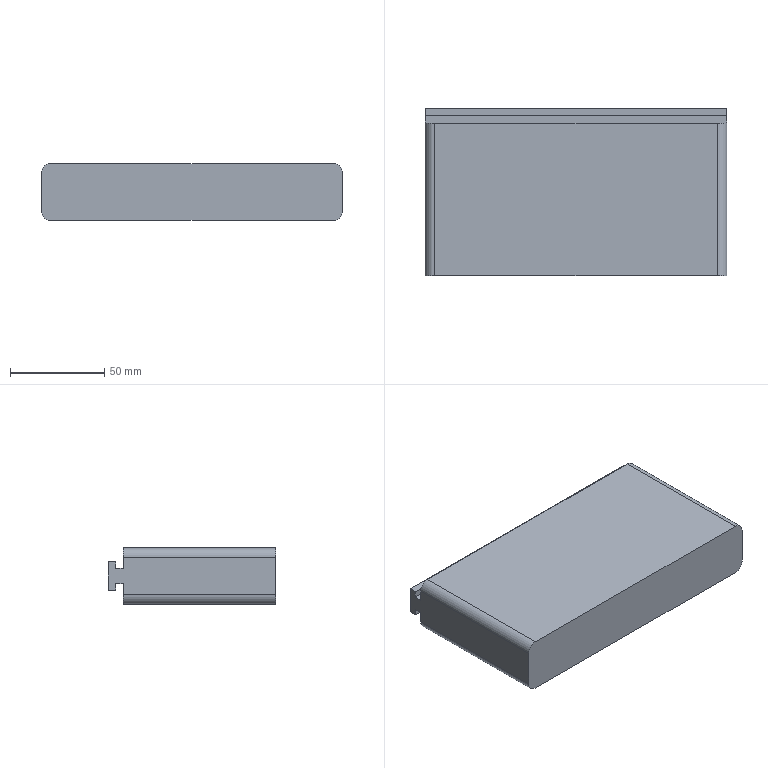Part | STEP file | RACK-BASE2_id654_x_t | 1 solid | 18 faces | box 160 x 89.028 x 30 mm | volume 401916 mm3 | plane 14 | cylinder 4 | commonest cylinder face diameters 10 x4
STEP:
#1=CARTESIAN_POINT('',(-110.,-174.472,83.5));
#2=VERTEX_POINT('',#1);
#3=CARTESIAN_POINT('',(50.,-174.472,83.5));
#4=VERTEX_POINT('',#3);
#5=CARTESIAN_POINT('',(30.,-174.472,83.5));
#6=DIRECTION('',(1.,0.,0.));
#7=VECTOR('',#6,1.);
#8=LINE('',#5,#7);
#9=EDGE_CURVE('',#2,#4,#8,.T.);
#10=ORIENTED_EDGE('',*,*,#9,.T.);
#11=CARTESIAN_POINT('',(50.,-174.472,77.5));
#12=VERTEX_POINT('',#11);
#13=CARTESIAN_POINT('',(50.,-174.472,102.5));
#14=DIRECTION('',(0.,0.,1.));
#15=VECTOR('',#14,1.);
#16=LINE('',#13,#15);
#17=EDGE_CURVE('',#12,#4,#16,.T.);
#18=ORIENTED_EDGE('',*,*,#17,.F.);
#19=CARTESIAN_POINT('',(45.,-174.472,72.5));
#20=VERTEX_POINT('',#19);
#21=CARTESIAN_POINT('',(45.,-174.472,77.5));
#22=DIRECTION('',(0.,-1.,0.));
#23=DIRECTION('',(0.,0.,-1.));
#24=AXIS2_PLACEMENT_3D('',#21,#22,#23);
#25=CIRCLE('',#24,5.);
#26=EDGE_CURVE('',#20,#12,#25,.T.);
#27=ORIENTED_EDGE('',*,*,#26,.F.);
#28=CARTESIAN_POINT('',(-105.,-174.472,72.5));
#29=VERTEX_POINT('',#28);
#30=CARTESIAN_POINT('',(50.126,-174.472,72.5));
#31=DIRECTION('',(1.,0.,0.));
#32=VECTOR('',#31,1.);
#33=LINE('',#30,#32);
#34=EDGE_CURVE('',#29,#20,#33,.T.);
#35=ORIENTED_EDGE('',*,*,#34,.F.);
#36=CARTESIAN_POINT('',(-110.,-174.472,77.5));
#37=VERTEX_POINT('',#36);
#38=CARTESIAN_POINT('',(-105.,-174.472,77.5));
#39=DIRECTION('',(0.,-1.,0.));
#40=DIRECTION('',(0.,0.,1.));
#41=AXIS2_PLACEMENT_3D('',#38,#39,#40);
#42=CIRCLE('',#41,5.);
#43=EDGE_CURVE('',#37,#29,#42,.T.);
#44=ORIENTED_EDGE('',*,*,#43,.F.);
#45=CARTESIAN_POINT('',(-110.,-174.472,102.5));
#46=DIRECTION('',(0.,0.,-1.));
#47=VECTOR('',#46,1.);
#48=LINE('',#45,#47);
#49=EDGE_CURVE('',#2,#37,#48,.T.);
#50=ORIENTED_EDGE('',*,*,#49,.F.);
#51=EDGE_LOOP('',(#10,#18,#27,#35,#44,#50));
#52=FACE_OUTER_BOUND('',#51,.T.);
#53=CARTESIAN_POINT('',(30.,-174.472,83.5));
#54=DIRECTION('',(0.,-1.,0.));
#55=DIRECTION('',(0.,0.,-1.));
#56=AXIS2_PLACEMENT_3D('',#53,#54,#55);
#57=PLANE('',#56);
#58=ADVANCED_FACE('',(#52),#57,.F.);
#59=CARTESIAN_POINT('',(-110.,-170.472,83.5));
#60=VERTEX_POINT('',#59);
#61=CARTESIAN_POINT('',(-110.,-255.5,83.5));
#62=DIRECTION('',(0.,-1.,0.));
#63=VECTOR('',#62,1.);
#64=LINE('',#61,#63);
#65=EDGE_CURVE('',#60,#2,#64,.T.);
#66=ORIENTED_EDGE('',*,*,#65,.F.);
#67=CARTESIAN_POINT('',(50.,-170.472,83.5));
#68=VERTEX_POINT('',#67);
#69=CARTESIAN_POINT('',(30.,-170.472,83.5));
#70=DIRECTION('',(1.,0.,0.));
#71=VECTOR('',#70,1.);
#72=LINE('',#69,#71);
#73=EDGE_CURVE('',#60,#68,#72,.T.);
#74=ORIENTED_EDGE('',*,*,#73,.T.);
#75=CARTESIAN_POINT('',(50.,-166.472,83.5));
#76=DIRECTION('',(0.,1.,0.));
#77=VECTOR('',#76,1.);
#78=LINE('',#75,#77);
#79=EDGE_CURVE('',#4,#68,#78,.T.);
#80=ORIENTED_EDGE('',*,*,#79,.F.);
#81=ORIENTED_EDGE('',*,*,#9,.F.);
#82=EDGE_LOOP('',(#66,#74,#80,#81));
#83=FACE_OUTER_BOUND('',#82,.T.);
#84=CARTESIAN_POINT('',(30.,-170.472,83.5));
#85=DIRECTION('',(0.,0.,1.));
#86=DIRECTION('',(1.,0.,0.));
#87=AXIS2_PLACEMENT_3D('',#84,#85,#86);
#88=PLANE('',#87);
#89=ADVANCED_FACE('',(#83),#88,.F.);
#90=CARTESIAN_POINT('',(-110.,-170.472,80.));
#91=VERTEX_POINT('',#90);
#92=CARTESIAN_POINT('',(-110.,-170.472,102.5));
#93=DIRECTION('',(0.,0.,1.));
#94=VECTOR('',#93,1.);
#95=LINE('',#92,#94);
#96=EDGE_CURVE('',#91,#60,#95,.T.);
#97=ORIENTED_EDGE('',*,*,#96,.F.);
#98=CARTESIAN_POINT('',(50.,-170.472,80.));
#99=VERTEX_POINT('',#98);
#100=CARTESIAN_POINT('',(30.,-170.472,80.));
#101=DIRECTION('',(1.,0.,0.));
#102=VECTOR('',#101,1.);
#103=LINE('',#100,#102);
#104=EDGE_CURVE('',#91,#99,#103,.T.);
#105=ORIENTED_EDGE('',*,*,#104,.T.);
#106=CARTESIAN_POINT('',(50.,-170.472,102.5));
#107=DIRECTION('',(0.,0.,-1.));
#108=VECTOR('',#107,1.);
#109=LINE('',#106,#108);
#110=EDGE_CURVE('',#68,#99,#109,.T.);
#111=ORIENTED_EDGE('',*,*,#110,.F.);
#112=ORIENTED_EDGE('',*,*,#73,.F.);
#113=EDGE_LOOP('',(#97,#105,#111,#112));
#114=FACE_OUTER_BOUND('',#113,.T.);
#115=CARTESIAN_POINT('',(30.,-170.472,80.));
#116=DIRECTION('',(0.,1.,0.));
#117=DIRECTION('',(0.,0.,1.));
#118=AXIS2_PLACEMENT_3D('',#115,#116,#117);
#119=PLANE('',#118);
#120=ADVANCED_FACE('',(#114),#119,.F.);
#121=CARTESIAN_POINT('',(-110.,-166.472,80.));
#122=VERTEX_POINT('',#121);
#123=CARTESIAN_POINT('',(-110.,-255.5,80.));
#124=DIRECTION('',(0.,-1.,0.));
#125=VECTOR('',#124,1.);
#126=LINE('',#123,#125);
#127=EDGE_CURVE('',#122,#91,#126,.T.);
#128=ORIENTED_EDGE('',*,*,#127,.F.);
#129=CARTESIAN_POINT('',(50.,-166.472,80.));
#130=VERTEX_POINT('',#129);
#131=CARTESIAN_POINT('',(-90.,-166.472,80.));
#132=DIRECTION('',(-1.,0.,0.));
#133=VECTOR('',#132,1.);
#134=LINE('',#131,#133);
#135=EDGE_CURVE('',#130,#122,#134,.T.);
#136=ORIENTED_EDGE('',*,*,#135,.F.);
#137=CARTESIAN_POINT('',(50.,-166.472,80.));
#138=DIRECTION('',(0.,1.,0.));
#139=VECTOR('',#138,1.);
#140=LINE('',#137,#139);
#141=EDGE_CURVE('',#99,#130,#140,.T.);
#142=ORIENTED_EDGE('',*,*,#141,.F.);
#143=ORIENTED_EDGE('',*,*,#104,.F.);
#144=EDGE_LOOP('',(#128,#136,#142,#143));
#145=FACE_OUTER_BOUND('',#144,.T.);
#146=CARTESIAN_POINT('',(30.,-166.472,80.));
#147=DIRECTION('',(0.,0.,1.));
#148=DIRECTION('',(1.,0.,0.));
#149=AXIS2_PLACEMENT_3D('',#146,#147,#148);
#150=PLANE('',#149);
#151=ADVANCED_FACE('',(#145),#150,.F.);
#152=CARTESIAN_POINT('',(-110.,-166.472,95.));
#153=VERTEX_POINT('',#152);
#154=CARTESIAN_POINT('',(-110.,-166.472,102.5));
#155=DIRECTION('',(0.,0.,-1.));
#156=VECTOR('',#155,1.);
#157=LINE('',#154,#156);
#158=EDGE_CURVE('',#153,#122,#157,.T.);
#159=ORIENTED_EDGE('',*,*,#158,.F.);
#160=CARTESIAN_POINT('',(50.,-166.472,95.));
#161=VERTEX_POINT('',#160);
#162=CARTESIAN_POINT('',(30.,-166.472,95.));
#163=DIRECTION('',(1.,0.,0.));
#164=VECTOR('',#163,1.);
#165=LINE('',#162,#164);
#166=EDGE_CURVE('',#153,#161,#165,.T.);
#167=ORIENTED_EDGE('',*,*,#166,.T.);
#168=CARTESIAN_POINT('',(50.,-166.472,102.5));
#169=DIRECTION('',(0.,0.,1.));
#170=VECTOR('',#169,1.);
#171=LINE('',#168,#170);
#172=EDGE_CURVE('',#130,#161,#171,.T.);
#173=ORIENTED_EDGE('',*,*,#172,.F.);
#174=ORIENTED_EDGE('',*,*,#135,.T.);
#175=EDGE_LOOP('',(#159,#167,#173,#174));
#176=FACE_OUTER_BOUND('',#175,.T.);
#177=CARTESIAN_POINT('',(-90.,-166.472,102.5));
#178=DIRECTION('',(0.,1.,0.));
#179=DIRECTION('',(0.,0.,1.));
#180=AXIS2_PLACEMENT_3D('',#177,#178,#179);
#181=PLANE('',#180);
#182=ADVANCED_FACE('',(#176),#181,.T.);
#183=CARTESIAN_POINT('',(-110.,-170.472,95.));
#184=VERTEX_POINT('',#183);
#185=CARTESIAN_POINT('',(-110.,-255.5,95.));
#186=DIRECTION('',(0.,1.,0.));
#187=VECTOR('',#186,1.);
#188=LINE('',#185,#187);
#189=EDGE_CURVE('',#184,#153,#188,.T.);
#190=ORIENTED_EDGE('',*,*,#189,.F.);
#191=CARTESIAN_POINT('',(50.,-170.472,95.));
#192=VERTEX_POINT('',#191);
#193=CARTESIAN_POINT('',(30.,-170.472,95.));
#194=DIRECTION('',(1.,0.,0.));
#195=VECTOR('',#194,1.);
#196=LINE('',#193,#195);
#197=EDGE_CURVE('',#184,#192,#196,.T.);
#198=ORIENTED_EDGE('',*,*,#197,.T.);
#199=CARTESIAN_POINT('',(50.,-166.472,95.));
#200=DIRECTION('',(0.,-1.,0.));
#201=VECTOR('',#200,1.);
#202=LINE('',#199,#201);
#203=EDGE_CURVE('',#161,#192,#202,.T.);
#204=ORIENTED_EDGE('',*,*,#203,.F.);
#205=ORIENTED_EDGE('',*,*,#166,.F.);
#206=EDGE_LOOP('',(#190,#198,#204,#205));
#207=FACE_OUTER_BOUND('',#206,.T.);
#208=CARTESIAN_POINT('',(30.,-170.472,95.));
#209=DIRECTION('',(0.,0.,-1.));
#210=DIRECTION('',(-1.,0.,0.));
#211=AXIS2_PLACEMENT_3D('',#208,#209,#210);
#212=PLANE('',#211);
#213=ADVANCED_FACE('',(#207),#212,.F.);
#214=CARTESIAN_POINT('',(-110.,-170.472,91.5));
#215=VERTEX_POINT('',#214);
#216=CARTESIAN_POINT('',(-110.,-170.472,102.5));
#217=DIRECTION('',(0.,0.,1.));
#218=VECTOR('',#217,1.);
#219=LINE('',#216,#218);
#220=EDGE_CURVE('',#215,#184,#219,.T.);
#221=ORIENTED_EDGE('',*,*,#220,.F.);
#222=CARTESIAN_POINT('',(50.,-170.472,91.5));
#223=VERTEX_POINT('',#222);
#224=CARTESIAN_POINT('',(30.,-170.472,91.5));
#225=DIRECTION('',(1.,0.,0.));
#226=VECTOR('',#225,1.);
#227=LINE('',#224,#226);
#228=EDGE_CURVE('',#215,#223,#227,.T.);
#229=ORIENTED_EDGE('',*,*,#228,.T.);
#230=CARTESIAN_POINT('',(50.,-170.472,102.5));
#231=DIRECTION('',(0.,0.,-1.));
#232=VECTOR('',#231,1.);
#233=LINE('',#230,#232);
#234=EDGE_CURVE('',#192,#223,#233,.T.);
#235=ORIENTED_EDGE('',*,*,#234,.F.);
#236=ORIENTED_EDGE('',*,*,#197,.F.);
#237=EDGE_LOOP('',(#221,#229,#235,#236));
#238=FACE_OUTER_BOUND('',#237,.T.);
#239=CARTESIAN_POINT('',(30.,-170.472,91.5));
#240=DIRECTION('',(0.,1.,0.));
#241=DIRECTION('',(0.,0.,1.));
#242=AXIS2_PLACEMENT_3D('',#239,#240,#241);
#243=PLANE('',#242);
#244=ADVANCED_FACE('',(#238),#243,.F.);
#245=CARTESIAN_POINT('',(-110.,-174.472,91.5));
#246=VERTEX_POINT('',#245);
#247=CARTESIAN_POINT('',(-110.,-255.5,91.5));
#248=DIRECTION('',(0.,1.,0.));
#249=VECTOR('',#248,1.);
#250=LINE('',#247,#249);
#251=EDGE_CURVE('',#246,#215,#250,.T.);
#252=ORIENTED_EDGE('',*,*,#251,.F.);
#253=CARTESIAN_POINT('',(50.,-174.472,91.5));
#254=VERTEX_POINT('',#253);
#255=CARTESIAN_POINT('',(30.,-174.472,91.5));
#256=DIRECTION('',(1.,0.,0.));
#257=VECTOR('',#256,1.);
#258=LINE('',#255,#257);
#259=EDGE_CURVE('',#246,#254,#258,.T.);
#260=ORIENTED_EDGE('',*,*,#259,.T.);
#261=CARTESIAN_POINT('',(50.,-166.472,91.5));
#262=DIRECTION('',(0.,-1.,0.));
#263=VECTOR('',#262,1.);
#264=LINE('',#261,#263);
#265=EDGE_CURVE('',#223,#254,#264,.T.);
#266=ORIENTED_EDGE('',*,*,#265,.F.);
#267=ORIENTED_EDGE('',*,*,#228,.F.);
#268=EDGE_LOOP('',(#252,#260,#266,#267));
#269=FACE_OUTER_BOUND('',#268,.T.);
#270=CARTESIAN_POINT('',(30.,-174.472,91.5));
#271=DIRECTION('',(0.,0.,-1.));
#272=DIRECTION('',(-1.,0.,0.));
#273=AXIS2_PLACEMENT_3D('',#270,#271,#272);
#274=PLANE('',#273);
#275=ADVANCED_FACE('',(#269),#274,.F.);
#276=CARTESIAN_POINT('',(-110.,-255.5,97.5));
#277=VERTEX_POINT('',#276);
#278=CARTESIAN_POINT('',(-110.,-255.5,77.5));
#279=VERTEX_POINT('',#278);
#280=CARTESIAN_POINT('',(-110.,-255.5,102.5));
#281=DIRECTION('',(0.,0.,-1.));
#282=VECTOR('',#281,1.);
#283=LINE('',#280,#282);
#284=EDGE_CURVE('',#277,#279,#283,.T.);
#285=ORIENTED_EDGE('',*,*,#284,.F.);
#286=CARTESIAN_POINT('',(-110.,-174.472,97.5));
#287=VERTEX_POINT('',#286);
#288=CARTESIAN_POINT('',(-110.,-174.182,97.5));
#289=DIRECTION('',(0.,-1.,0.));
#290=VECTOR('',#289,1.);
#291=LINE('',#288,#290);
#292=EDGE_CURVE('',#287,#277,#291,.T.);
#293=ORIENTED_EDGE('',*,*,#292,.F.);
#294=CARTESIAN_POINT('',(-110.,-174.472,102.5));
#295=DIRECTION('',(0.,0.,-1.));
#296=VECTOR('',#295,1.);
#297=LINE('',#294,#296);
#298=EDGE_CURVE('',#287,#246,#297,.T.);
#299=ORIENTED_EDGE('',*,*,#298,.T.);
#300=ORIENTED_EDGE('',*,*,#251,.T.);
#301=ORIENTED_EDGE('',*,*,#220,.T.);
#302=ORIENTED_EDGE('',*,*,#189,.T.);
#303=ORIENTED_EDGE('',*,*,#158,.T.);
#304=ORIENTED_EDGE('',*,*,#127,.T.);
#305=ORIENTED_EDGE('',*,*,#96,.T.);
#306=ORIENTED_EDGE('',*,*,#65,.T.);
#307=ORIENTED_EDGE('',*,*,#49,.T.);
#308=CARTESIAN_POINT('',(-110.,-255.78,77.5));
#309=DIRECTION('',(0.,1.,0.));
#310=VECTOR('',#309,1.);
#311=LINE('',#308,#310);
#312=EDGE_CURVE('',#279,#37,#311,.T.);
#313=ORIENTED_EDGE('',*,*,#312,.F.);
#314=EDGE_LOOP('',(#285,#293,#299,#300,#301,#302,#303,#304,#305,#306,#307,#313));
#315=FACE_OUTER_BOUND('',#314,.T.);
#316=CARTESIAN_POINT('',(-110.,-255.5,102.5));
#317=DIRECTION('',(-1.,0.,0.));
#318=DIRECTION('',(0.,0.,1.));
#319=AXIS2_PLACEMENT_3D('',#316,#317,#318);
#320=PLANE('',#319);
#321=ADVANCED_FACE('',(#315),#320,.T.);
#322=CARTESIAN_POINT('',(-105.,-255.5,72.5));
#323=VERTEX_POINT('',#322);
#324=CARTESIAN_POINT('',(-105.,-255.5,77.5));
#325=DIRECTION('',(0.,-1.,0.));
#326=DIRECTION('',(0.,0.,1.));
#327=AXIS2_PLACEMENT_3D('',#324,#325,#326);
#328=CIRCLE('',#327,5.);
#329=EDGE_CURVE('',#279,#323,#328,.T.);
#330=ORIENTED_EDGE('',*,*,#329,.F.);
#331=ORIENTED_EDGE('',*,*,#312,.T.);
#332=ORIENTED_EDGE('',*,*,#43,.T.);
#333=CARTESIAN_POINT('',(-105.,-0.5,72.5));
#334=DIRECTION('',(0.,1.,0.));
#335=VECTOR('',#334,1.);
#336=LINE('',#333,#335);
#337=EDGE_CURVE('',#323,#29,#336,.T.);
#338=ORIENTED_EDGE('',*,*,#337,.F.);
#339=EDGE_LOOP('',(#330,#331,#332,#338));
#340=FACE_OUTER_BOUND('',#339,.T.);
#341=CARTESIAN_POINT('',(-105.,-255.78,77.5));
#342=DIRECTION('',(0.,1.,0.));
#343=DIRECTION('',(0.,0.,1.));
#344=AXIS2_PLACEMENT_3D('',#341,#342,#343);
#345=CYLINDRICAL_SURFACE('',#344,5.);
#346=ADVANCED_FACE('',(#340),#345,.T.);
#347=CARTESIAN_POINT('',(45.,-255.5,72.5));
#348=VERTEX_POINT('',#347);
#349=CARTESIAN_POINT('',(30.,-255.5,72.5));
#350=DIRECTION('',(1.,0.,0.));
#351=VECTOR('',#350,1.);
#352=LINE('',#349,#351);
#353=EDGE_CURVE('',#323,#348,#352,.T.);
#354=ORIENTED_EDGE('',*,*,#353,.F.);
#355=ORIENTED_EDGE('',*,*,#337,.T.);
#356=ORIENTED_EDGE('',*,*,#34,.T.);
#357=CARTESIAN_POINT('',(45.,-174.182,72.5));
#358=DIRECTION('',(0.,1.,0.));
#359=VECTOR('',#358,1.);
#360=LINE('',#357,#359);
#361=EDGE_CURVE('',#348,#20,#360,.T.);
#362=ORIENTED_EDGE('',*,*,#361,.F.);
#363=EDGE_LOOP('',(#354,#355,#356,#362));
#364=FACE_OUTER_BOUND('',#363,.T.);
#365=CARTESIAN_POINT('',(50.126,-0.5,72.5));
#366=DIRECTION('',(0.,0.,-1.));
#367=DIRECTION('',(-1.,0.,0.));
#368=AXIS2_PLACEMENT_3D('',#365,#366,#367);
#369=PLANE('',#368);
#370=ADVANCED_FACE('',(#364),#369,.T.);
#371=ORIENTED_EDGE('',*,*,#26,.T.);
#372=CARTESIAN_POINT('',(50.,-255.5,77.5));
#373=VERTEX_POINT('',#372);
#374=CARTESIAN_POINT('',(50.,-166.472,77.5));
#375=DIRECTION('',(0.,1.,0.));
#376=VECTOR('',#375,1.);
#377=LINE('',#374,#376);
#378=EDGE_CURVE('',#373,#12,#377,.T.);
#379=ORIENTED_EDGE('',*,*,#378,.F.);
#380=CARTESIAN_POINT('',(45.,-255.5,77.5));
#381=DIRECTION('',(0.,-1.,0.));
#382=DIRECTION('',(0.,0.,-1.));
#383=AXIS2_PLACEMENT_3D('',#380,#381,#382);
#384=CIRCLE('',#383,5.);
#385=EDGE_CURVE('',#348,#373,#384,.T.);
#386=ORIENTED_EDGE('',*,*,#385,.F.);
#387=ORIENTED_EDGE('',*,*,#361,.T.);
#388=EDGE_LOOP('',(#371,#379,#386,#387));
#389=FACE_OUTER_BOUND('',#388,.T.);
#390=CARTESIAN_POINT('',(45.,-174.182,77.5));
#391=DIRECTION('',(0.,-1.,0.));
#392=DIRECTION('',(0.,0.,-1.));
#393=AXIS2_PLACEMENT_3D('',#390,#391,#392);
#394=CYLINDRICAL_SURFACE('',#393,5.);
#395=ADVANCED_FACE('',(#389),#394,.T.);
#396=CARTESIAN_POINT('',(50.,-174.472,97.5));
#397=VERTEX_POINT('',#396);
#398=CARTESIAN_POINT('',(50.,-174.472,102.5));
#399=DIRECTION('',(0.,0.,1.));
#400=VECTOR('',#399,1.);
#401=LINE('',#398,#400);
#402=EDGE_CURVE('',#254,#397,#401,.T.);
#403=ORIENTED_EDGE('',*,*,#402,.T.);
#404=CARTESIAN_POINT('',(50.,-255.5,97.5));
#405=VERTEX_POINT('',#404);
#406=CARTESIAN_POINT('',(50.,-255.78,97.5));
#407=DIRECTION('',(0.,1.,0.));
#408=VECTOR('',#407,1.);
#409=LINE('',#406,#408);
#410=EDGE_CURVE('',#405,#397,#409,.T.);
#411=ORIENTED_EDGE('',*,*,#410,.F.);
#412=CARTESIAN_POINT('',(50.,-255.5,102.5));
#413=DIRECTION('',(0.,0.,1.));
#414=VECTOR('',#413,1.);
#415=LINE('',#412,#414);
#416=EDGE_CURVE('',#373,#405,#415,.T.);
#417=ORIENTED_EDGE('',*,*,#416,.F.);
#418=ORIENTED_EDGE('',*,*,#378,.T.);
#419=ORIENTED_EDGE('',*,*,#17,.T.);
#420=ORIENTED_EDGE('',*,*,#79,.T.);
#421=ORIENTED_EDGE('',*,*,#110,.T.);
#422=ORIENTED_EDGE('',*,*,#141,.T.);
#423=ORIENTED_EDGE('',*,*,#172,.T.);
#424=ORIENTED_EDGE('',*,*,#203,.T.);
#425=ORIENTED_EDGE('',*,*,#234,.T.);
#426=ORIENTED_EDGE('',*,*,#265,.T.);
#427=EDGE_LOOP('',(#403,#411,#417,#418,#419,#420,#421,#422,#423,#424,#425,#426));
#428=FACE_OUTER_BOUND('',#427,.T.);
#429=CARTESIAN_POINT('',(50.,-166.472,102.5));
#430=DIRECTION('',(1.,0.,0.));
#431=DIRECTION('',(0.,0.,-1.));
#432=AXIS2_PLACEMENT_3D('',#429,#430,#431);
#433=PLANE('',#432);
#434=ADVANCED_FACE('',(#428),#433,.T.);
#435=CARTESIAN_POINT('',(-105.,-174.472,102.5));
#436=VERTEX_POINT('',#435);
#437=CARTESIAN_POINT('',(-105.,-174.472,97.5));
#438=DIRECTION('',(0.,-1.,0.));
#439=DIRECTION('',(0.,0.,-1.));
#440=AXIS2_PLACEMENT_3D('',#437,#438,#439);
#441=CIRCLE('',#440,5.);
#442=EDGE_CURVE('',#436,#287,#441,.T.);
#443=ORIENTED_EDGE('',*,*,#442,.T.);
#444=ORIENTED_EDGE('',*,*,#292,.T.);
#445=CARTESIAN_POINT('',(-105.,-255.5,102.5));
#446=VERTEX_POINT('',#445);
#447=CARTESIAN_POINT('',(-105.,-255.5,97.5));
#448=DIRECTION('',(0.,-1.,0.));
#449=DIRECTION('',(0.,0.,-1.));
#450=AXIS2_PLACEMENT_3D('',#447,#448,#449);
#451=CIRCLE('',#450,5.);
#452=EDGE_CURVE('',#446,#277,#451,.T.);
#453=ORIENTED_EDGE('',*,*,#452,.F.);
#454=CARTESIAN_POINT('',(-105.,0.,102.5));
#455=DIRECTION('',(0.,1.,0.));
#456=VECTOR('',#455,1.);
#457=LINE('',#454,#456);
#458=EDGE_CURVE('',#446,#436,#457,.T.);
#459=ORIENTED_EDGE('',*,*,#458,.T.);
#460=EDGE_LOOP('',(#443,#444,#453,#459));
#461=FACE_OUTER_BOUND('',#460,.T.);
#462=CARTESIAN_POINT('',(-105.,-174.182,97.5));
#463=DIRECTION('',(0.,-1.,0.));
#464=DIRECTION('',(0.,0.,-1.));
#465=AXIS2_PLACEMENT_3D('',#462,#463,#464);
#466=CYLINDRICAL_SURFACE('',#465,5.);
#467=ADVANCED_FACE('',(#461),#466,.T.);
#468=CARTESIAN_POINT('',(45.,-174.472,102.5));
#469=VERTEX_POINT('',#468);
#470=CARTESIAN_POINT('',(45.,-174.472,97.5));
#471=DIRECTION('',(0.,-1.,0.));
#472=DIRECTION('',(0.,0.,1.));
#473=AXIS2_PLACEMENT_3D('',#470,#471,#472);
#474=CIRCLE('',#473,5.);
#475=EDGE_CURVE('',#397,#469,#474,.T.);
#476=ORIENTED_EDGE('',*,*,#475,.F.);
#477=ORIENTED_EDGE('',*,*,#402,.F.);
#478=ORIENTED_EDGE('',*,*,#259,.F.);
#479=ORIENTED_EDGE('',*,*,#298,.F.);
#480=ORIENTED_EDGE('',*,*,#442,.F.);
#481=CARTESIAN_POINT('',(0.,-174.472,102.5));
#482=DIRECTION('',(1.,0.,0.));
#483=VECTOR('',#482,1.);
#484=LINE('',#481,#483);
#485=EDGE_CURVE('',#436,#469,#484,.T.);
#486=ORIENTED_EDGE('',*,*,#485,.T.);
#487=EDGE_LOOP('',(#476,#477,#478,#479,#480,#486));
#488=FACE_OUTER_BOUND('',#487,.T.);
#489=CARTESIAN_POINT('',(30.,-174.472,102.5));
#490=DIRECTION('',(0.,-1.,0.));
#491=DIRECTION('',(0.,0.,-1.));
#492=AXIS2_PLACEMENT_3D('',#489,#490,#491);
#493=PLANE('',#492);
#494=ADVANCED_FACE('',(#488),#493,.F.);
#495=CARTESIAN_POINT('',(45.,-255.5,102.5));
#496=VERTEX_POINT('',#495);
#497=CARTESIAN_POINT('',(45.,-255.5,97.5));
#498=DIRECTION('',(0.,-1.,0.));
#499=DIRECTION('',(0.,0.,1.));
#500=AXIS2_PLACEMENT_3D('',#497,#498,#499);
#501=CIRCLE('',#500,5.);
#502=EDGE_CURVE('',#405,#496,#501,.T.);
#503=ORIENTED_EDGE('',*,*,#502,.F.);
#504=ORIENTED_EDGE('',*,*,#410,.T.);
#505=ORIENTED_EDGE('',*,*,#475,.T.);
#506=CARTESIAN_POINT('',(45.,0.,102.5));
#507=DIRECTION('',(0.,-1.,0.));
#508=VECTOR('',#507,1.);
#509=LINE('',#506,#508);
#510=EDGE_CURVE('',#469,#496,#509,.T.);
#511=ORIENTED_EDGE('',*,*,#510,.T.);
#512=EDGE_LOOP('',(#503,#504,#505,#511));
#513=FACE_OUTER_BOUND('',#512,.T.);
#514=CARTESIAN_POINT('',(45.,-255.78,97.5));
#515=DIRECTION('',(0.,1.,0.));
#516=DIRECTION('',(0.,0.,1.));
#517=AXIS2_PLACEMENT_3D('',#514,#515,#516);
#518=CYLINDRICAL_SURFACE('',#517,5.);
#519=ADVANCED_FACE('',(#513),#518,.T.);
#520=CARTESIAN_POINT('',(0.,-255.5,102.5));
#521=DIRECTION('',(-1.,0.,0.));
#522=VECTOR('',#521,1.);
#523=LINE('',#520,#522);
#524=EDGE_CURVE('',#496,#446,#523,.T.);
#525=ORIENTED_EDGE('',*,*,#524,.T.);
#526=ORIENTED_EDGE('',*,*,#452,.T.);
#527=ORIENTED_EDGE('',*,*,#284,.T.);
#528=ORIENTED_EDGE('',*,*,#329,.T.);
#529=ORIENTED_EDGE('',*,*,#353,.T.);
#530=ORIENTED_EDGE('',*,*,#385,.T.);
#531=ORIENTED_EDGE('',*,*,#416,.T.);
#532=ORIENTED_EDGE('',*,*,#502,.T.);
#533=EDGE_LOOP('',(#525,#526,#527,#528,#529,#530,#531,#532));
#534=FACE_OUTER_BOUND('',#533,.T.);
#535=CARTESIAN_POINT('',(30.,-255.5,102.5));
#536=DIRECTION('',(0.,-1.,0.));
#537=DIRECTION('',(0.,0.,-1.));
#538=AXIS2_PLACEMENT_3D('',#535,#536,#537);
#539=PLANE('',#538);
#540=ADVANCED_FACE('',(#534),#539,.T.);
#541=ORIENTED_EDGE('',*,*,#510,.F.);
#542=ORIENTED_EDGE('',*,*,#485,.F.);
#543=ORIENTED_EDGE('',*,*,#458,.F.);
#544=ORIENTED_EDGE('',*,*,#524,.F.);
#545=EDGE_LOOP('',(#541,#542,#543,#544));
#546=FACE_OUTER_BOUND('',#545,.T.);
#547=CARTESIAN_POINT('',(0.,0.,102.5));
#548=DIRECTION('',(0.,0.,-1.));
#549=DIRECTION('',(-1.,0.,0.));
#550=AXIS2_PLACEMENT_3D('',#547,#548,#549);
#551=PLANE('',#550);
#552=ADVANCED_FACE('',(#546),#551,.F.);
#553=CLOSED_SHELL('',(#58,#89,#120,#151,#182,#213,#244,#275,#321,#346,#370,#395,#434,#467,#494,#519,#540,#552));
#554=MANIFOLD_SOLID_BREP('',#553);
#555=(LENGTH_UNIT()NAMED_UNIT(*)SI_UNIT(.MILLI.,.METRE.));
#556=UNCERTAINTY_MEASURE_WITH_UNIT(LENGTH_MEASURE(0.00004123),#555,'','');
#557=(NAMED_UNIT(*)PLANE_ANGLE_UNIT()SI_UNIT($,.RADIAN.));
#558=PLANE_ANGLE_MEASURE_WITH_UNIT(PLANE_ANGLE_MEASURE(0.01745),#557);
#559=DIMENSIONAL_EXPONENTS(0.,0.,0.,0.,0.,0.,0.);
#560=(CONVERSION_BASED_UNIT('DEGREE',#558)NAMED_UNIT(#559)PLANE_ANGLE_UNIT());
#561=(NAMED_UNIT(*)SI_UNIT($,.STERADIAN.)SOLID_ANGLE_UNIT());
#562=(GEOMETRIC_REPRESENTATION_CONTEXT(3)GLOBAL_UNCERTAINTY_ASSIGNED_CONTEXT((#556))GLOBAL_UNIT_ASSIGNED_CONTEXT((#555,#560,#561))REPRESENTATION_CONTEXT('',''));
#563=ADVANCED_BREP_SHAPE_REPRESENTATION('',(#554),#562);